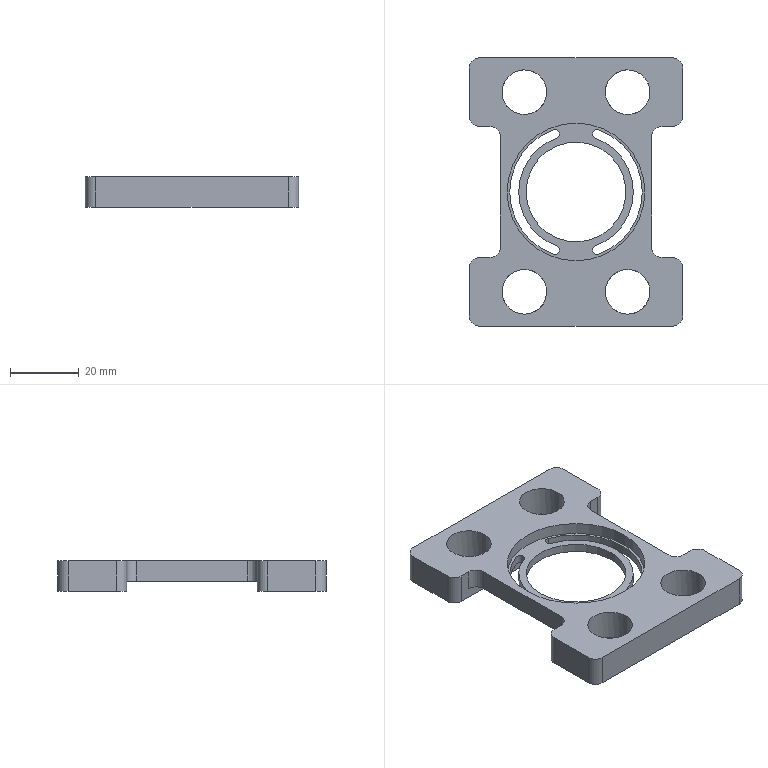NC program | NX | posted with a generic post | part box 62 x 78 x 9 mm
Whole program:
N10 G17 G21 G94 G90
(FLOOR_WALL_COPY , TOOL : D10)
N12 T10 M6
N14 G54
N16 G17 G0 G90 X-47. Y30.997 S9500 M3
N18 G43 Z30. H10
N20 Z3.
N22 G94 G1 Z0. F1250.
N24 X-44.
N26 X44.
N28 Y26.164
N30 X-44.
N32 Y21.331
N34 X44.
N36 Y16.498
N38 X-44.
N40 Y11.665
N42 X44.
N44 Y6.832
N46 X-44.
N48 Y1.999
N50 X44.
N52 Y-2.835
N54 X-44.
N56 Y-7.668
N58 X44.
N60 Y-12.501
N62 X-44.
N64 Y-17.334
N66 X44.
N68 Y-22.167
N70 X-44.
N72 Y-27.
N74 X44.
N76 X47.
N78 Z3.
N80 G0 Z30.
(FLOOR_WALL_COPY_COPY , TOOL : D10)
N82 X13.897 Y35.586
N84 Z2.517
N86 G1 Z-0.483 F2500.
N88 Y27.
N90 Y-27.
N92 X9.264
N94 Y27.
N96 X4.631
N98 Y-27.
N100 X-0.001
N102 Y27.
N104 X-4.634
N106 Y-27.
N108 X-9.267
N110 Y27.
N112 X-13.9
N114 Y-27.
N116 Y-35.589
N118 Z2.517
N120 G0 Z30.
N122 X13.897 Y35.586
N124 Z2.033
N126 G1 Z-0.967
N128 Y27.
N130 Y-27.
N132 X9.264
N134 Y27.
N136 X4.631
N138 Y-27.
N140 X-0.001
N142 Y27.
N144 X-4.634
N146 Y-27.
N148 X-9.267
N150 Y27.
N152 X-13.9
N154 Y-27.
N156 Y-35.589
N158 Z2.033
N160 G0 Z30.
N162 X13.897 Y35.586
N164 Z1.55
N166 G1 Z-1.45
N168 Y27.
N170 Y-27.
N172 X9.264
N174 Y27.
N176 X4.631
N178 Y-27.
N180 X-0.001
N182 Y27.
N184 X-4.634
N186 Y-27.
N188 X-9.267
N190 Y27.
N192 X-13.9
N194 Y-27.
N196 Y-35.589
N198 Z1.55
N200 G0 Z30.
N202 X13.897 Y35.586
N204 Z1.067
N206 G1 Z-1.933
N208 Y27.
N210 Y-27.
N212 X9.264
N214 Y27.
N216 X4.631
N218 Y-27.
N220 X-0.001
N222 Y27.
N224 X-4.634
N226 Y-27.
N228 X-9.267
N230 Y27.
N232 X-13.9
N234 Y-27.
N236 Y-35.589
N238 Z1.067
N240 G0 Z30.
N242 X13.897 Y35.586
N244 Z0.583
N246 G1 Z-2.417
N248 Y27.
N250 Y-27.
N252 X9.264
N254 Y27.
N256 X4.631
N258 Y-27.
N260 X-0.001
N262 Y27.
N264 X-4.634
N266 Y-27.
N268 X-9.267
N270 Y27.
N272 X-13.9
N274 Y-27.
N276 Y-35.589
N278 Z0.583
N280 G0 Z30.
N282 X13.897 Y35.586
N284 Z0.1
N286 G1 Z-2.9
N288 Y27.
N290 Y-27.
N292 X9.264
N294 Y27.
N296 X4.631
N298 Y-27.
N300 X-0.001
N302 Y27.
N304 X-4.634
N306 Y-27.
N308 X-9.267
N310 Y27.
N312 X-13.9
N314 Y-27.
N316 Y-35.589
N318 Z0.1
N320 G0 Z30.
(FLOOR_WALL_COPY_COPY_COPY , TOOL : D10)
N322 X13.497 Y34.978
N324 Z0.
N326 G1 Z-3. F1200.
N328 Y27.
N330 Y-27.
N332 X8.998
N334 Y27.
N336 X4.498
N338 Y-27.
N340 X-0.001
N342 Y27.
N344 X-4.501
N346 Y-27.
N348 X-9.
N350 Y27.
N352 X-13.5
N354 Y-27.
N356 Y-34.982
N358 Z0.
N360 G0 Z30.
N362 X14. Y-35.55
N364 Z0.
N366 G1 Z-3.
N368 Y-27.
N370 Y26.97
N372 Y35.55
N374 Z0.
N376 G0 Z30.
N378 X-14.
N380 Z0.
N382 G1 Z-3.
N384 Y27.
N386 Y-26.97
N388 Y-35.55
N390 Z0.
N392 G0 Z30.
N394 M5
(PLANAR_MILL_COPY_1 , TOOL : D6A45)
N396 T07 M6
N398 G54
N400 G17 G0 G90 X-34.243 Y15.766 S9500 M3
N402 G43 Z30. H7
N404 Z0.
N406 G94 G1 Z-1. F1250.
N408 G3 X-34.6 Y15. R1.
N410 X-29. Y9.4 R5.6
N412 X-34.6 Y15. R-5.6
N414 X-34.243 Y14.234 R1.
N416 G1 Z0.
N418 G0 Z30.
N420 X-40.257 Y-0.766
N422 Z0.
N424 G1 Z-1.
N426 G3 X-39.9 Y0. R1.
N428 G1 Y28.
N430 G2 X-36. Y31.9 R3.9
N432 G1 X-22.
N434 G2 X-18.1 Y28. R3.9
N436 G1 Y-28.
N438 G2 X-22. Y-31.9 R3.9
N440 G1 X-36.
N442 G2 X-39.9 Y-28. R3.9
N444 G1 Y0.
N446 G3 X-40.257 Y0.766 R1.
N448 G1 Z0.
N450 G0 Z30.
N452 X-34.243 Y-14.234
N454 Z0.
N456 G1 Z-1.
N458 G3 X-34.6 Y-15. R1.
N460 X-29. Y-20.6 R5.6
N462 X-34.6 Y-15. R-5.6
N464 X-34.243 Y-15.766 R1.
N466 G1 Z0.
N468 G0 Z30.
N470 X34.243
N472 Z0.
N474 G1 Z-1.
N476 G3 X34.6 Y-15. R1.
N478 X29. Y-9.4 R5.6
N480 X34.6 Y-15. R-5.6
N482 X34.243 Y-14.234 R1.
N484 G1 Z0.
N486 G0 Z30.
N488 X40.257 Y0.766
N490 Z0.
N492 G1 Z-1.
N494 G3 X39.9 Y0. R1.
N496 G1 Y-28.
N498 G2 X36. Y-31.9 R3.9
N500 G1 X22.
N502 G2 X18.1 Y-28. R3.9
N504 G1 Y28.
N506 G2 X22. Y31.9 R3.9
N508 G1 X36.
N510 G2 X39.9 Y28. R3.9
N512 G1 Y0.
N514 G3 X40.257 Y-0.766 R1.
N516 G1 Z0.
N518 G0 Z30.
N520 X34.243 Y14.234
N522 Z0.
N524 G1 Z-1.
N526 G3 X34.6 Y15. R1.
N528 X29. Y20.6 R5.6
N530 X34.6 Y15. R-5.6
N532 X34.243 Y15.766 R1.
N534 G1 Z0.
N536 G0 Z30.
(PLANAR_MILL_COPY_1_COPY , TOOL : D6A45)
N538 X-13.208 Y-12.759
N540 Z-3.
N542 G1 X-14.938 Y-10.709 Z-3.719
N544 X-15.5 Y-9.822 Z-4.
N546 G3 X15.5 Y-9.822 R18.35
N548 X15.143 Y-9.056 R1.
N550 G1 Y-8.997
N552 G3 X15.5 Y-8.231 R1.
N554 G2 X-15.5 Y-8.231 R17.55
N556 G3 X-15.143 Y-8.997 R1.
N558 G1 Z-3.
N560 G0 Z30.
N562 X-1.555 Y-12.302
N564 Z-3.
N566 G1 Z-4.
N568 X-0.766 Y-13.243
N570 G3 X0. Y-13.6 R1.
N572 X13.6 Y0. R13.6
N574 X0. Y-13.6 R-13.6
N576 X0.766 Y-13.243 R1.
N578 G1 X1.555 Y-12.302
N580 Z-3.
N582 G0 Z30.
N584 X14.3 Y-24.373
N586 Z-3.
N588 G1 Z-4.
N590 X15.143 Y-23.666
N592 G3 X15.5 Y-22.9 R1.
N594 G1 X-15.5
N596 G3 X-15.143 Y-23.666 R1.
N598 G1 X-14.3 Y-24.373
N600 Z-3.
N602 G0 Z30.
N604 Y24.373
N606 Z-3.
N608 G1 Z-4.
N610 X-15.143 Y23.666
N612 G3 X-15.5 Y22.9 R1.
N614 G1 X15.5
N616 G3 X15.143 Y23.666 R1.
N618 G1 X14.3 Y24.373
N620 Z-3.
N622 G0 Z30.
N624 X13.208 Y12.759
N626 Z-3.
N628 G1 X14.938 Y10.709 Z-3.719
N630 X15.5 Y9.822 Z-4.
N632 G3 X-15.5 Y9.822 R18.35
N634 X-15.143 Y9.056 R1.
N636 G1 Y8.997
N638 G3 X-15.5 Y8.231 R1.
N640 G2 X15.5 Y8.231 R17.55
N642 G3 X15.143 Y8.997 R1.
N644 G1 Z-3.
N646 G0 Z30.
N648 M5
N650 M2